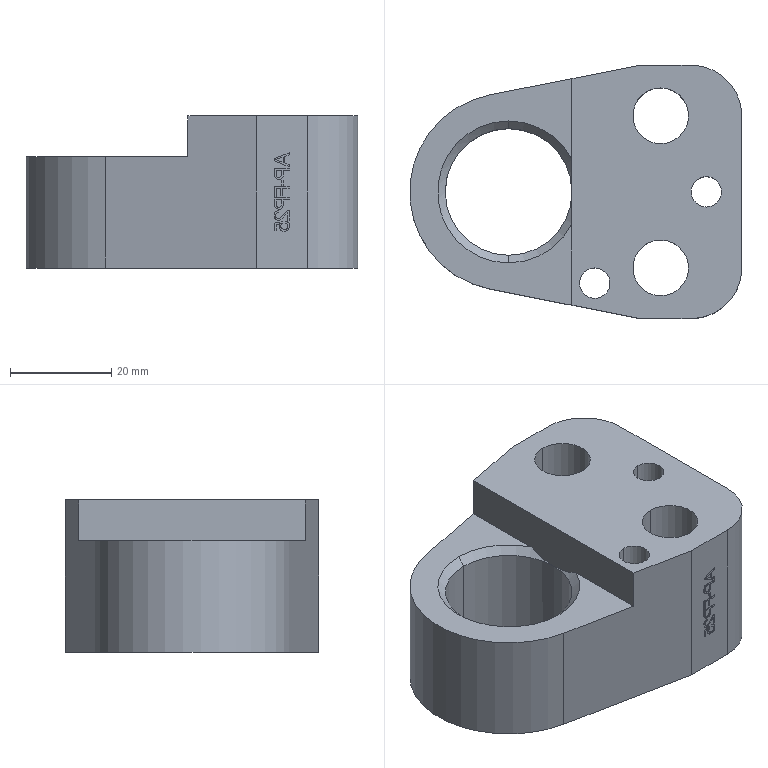Part | NX | features AP-FP25_8 2 | 1 solid | 127 faces | box 65.5 x 50 x 30 mm | volume 49937 mm3 | plane 83 | cylinder 40 | cone 4 | commonest cylinder face diameters 6 x4 6.8 x4 8 x4 11 x4 17 x4 1.055 x2